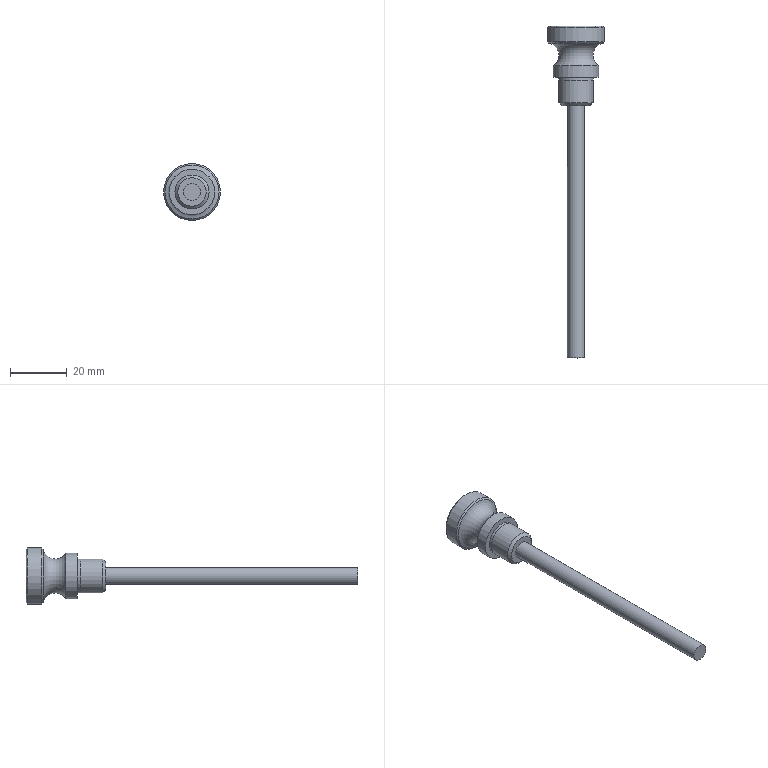Part | NX | 1 solid | 14 faces | box 20.002 x 116.72 x 20.002 mm | volume 7452 mm3 | plane 5 | cone 4 | cylinder 4 | torus 1 | commonest cylinder face diameters 5.996 x1 12.002 x1 16.002 x1 20.002 x1
STEP:
#1=CARTESIAN_POINT('',(9.502,116.719,0.));
#2=VERTEX_POINT('',#1);
#3=CARTESIAN_POINT('',(0.000965,116.72,0.));
#4=DIRECTION('',(-0.000008268,-1.,0.));
#5=DIRECTION('',(1.,-0.000008268,0.));
#6=AXIS2_PLACEMENT_3D('',#3,#4,#5);
#7=CIRCLE('',#6,9.501);
#8=EDGE_CURVE('',#2,#2,#7,.T.);
#9=ORIENTED_EDGE('',*,*,#8,.F.);
#10=EDGE_LOOP('',(#9));
#11=FACE_OUTER_BOUND('',#10,.T.);
#12=CARTESIAN_POINT('',(-9.5,116.72,0.));
#13=DIRECTION('',(0.000008268,1.,0.));
#14=DIRECTION('',(1.,-0.000008268,0.));
#15=AXIS2_PLACEMENT_3D('',#12,#13,#14);
#16=PLANE('',#15);
#17=ADVANCED_FACE('',(#11),#16,.T.);
#18=ORIENTED_EDGE('',*,*,#8,.T.);
#19=EDGE_LOOP('',(#18));
#20=FACE_BOUND('',#19,.T.);
#21=CARTESIAN_POINT('',(10.002,116.219,0.));
#22=VERTEX_POINT('',#21);
#23=CARTESIAN_POINT('',(0.0009609,116.22,0.));
#24=DIRECTION('',(-0.000008268,-1.,0.));
#25=DIRECTION('',(1.,-0.000008268,0.));
#26=AXIS2_PLACEMENT_3D('',#23,#24,#25);
#27=CIRCLE('',#26,10.001);
#28=EDGE_CURVE('',#22,#22,#27,.T.);
#29=ORIENTED_EDGE('',*,*,#28,.F.);
#30=EDGE_LOOP('',(#29));
#31=FACE_BOUND('',#30,.T.);
#32=CARTESIAN_POINT('',(0.0009609,116.22,0.));
#33=DIRECTION('',(-0.000008268,-1.,0.));
#34=DIRECTION('',(-1.,0.000008268,0.));
#35=AXIS2_PLACEMENT_3D('',#32,#33,#34);
#36=CONICAL_SURFACE('',#35,10.001,45.);
#37=ADVANCED_FACE('',(#20,#31),#36,.T.);
#38=ORIENTED_EDGE('',*,*,#28,.T.);
#39=EDGE_LOOP('',(#38));
#40=FACE_BOUND('',#39,.T.);
#41=CARTESIAN_POINT('',(10.002,111.219,0.));
#42=VERTEX_POINT('',#41);
#43=CARTESIAN_POINT('',(0.0009195,111.22,0.));
#44=DIRECTION('',(-0.000008268,-1.,0.));
#45=DIRECTION('',(1.,-0.000008268,0.));
#46=AXIS2_PLACEMENT_3D('',#43,#44,#45);
#47=CIRCLE('',#46,10.001);
#48=EDGE_CURVE('',#42,#42,#47,.T.);
#49=ORIENTED_EDGE('',*,*,#48,.F.);
#50=EDGE_LOOP('',(#49));
#51=FACE_BOUND('',#50,.T.);
#52=CARTESIAN_POINT('',(-0.00004139,-5.006,0.));
#53=DIRECTION('',(-0.000008268,-1.,0.));
#54=DIRECTION('',(-1.,0.000008268,0.));
#55=AXIS2_PLACEMENT_3D('',#52,#53,#54);
#56=CYLINDRICAL_SURFACE('',#55,10.001);
#57=ADVANCED_FACE('',(#40,#51),#56,.T.);
#58=ORIENTED_EDGE('',*,*,#48,.T.);
#59=EDGE_LOOP('',(#58));
#60=FACE_BOUND('',#59,.T.);
#61=CARTESIAN_POINT('',(9.502,110.719,0.));
#62=VERTEX_POINT('',#61);
#63=CARTESIAN_POINT('',(0.0009154,110.72,0.));
#64=DIRECTION('',(-0.000008268,-1.,0.));
#65=DIRECTION('',(1.,-0.000008268,0.));
#66=AXIS2_PLACEMENT_3D('',#63,#64,#65);
#67=CIRCLE('',#66,9.501);
#68=EDGE_CURVE('',#62,#62,#67,.T.);
#69=ORIENTED_EDGE('',*,*,#68,.F.);
#70=EDGE_LOOP('',(#69));
#71=FACE_BOUND('',#70,.T.);
#72=CARTESIAN_POINT('',(0.0009154,110.72,0.));
#73=DIRECTION('',(0.000008268,1.,0.));
#74=DIRECTION('',(1.,-0.000008268,0.));
#75=AXIS2_PLACEMENT_3D('',#72,#73,#74);
#76=CONICAL_SURFACE('',#75,9.501,45.);
#77=ADVANCED_FACE('',(#60,#71),#76,.T.);
#78=ORIENTED_EDGE('',*,*,#68,.T.);
#79=EDGE_LOOP('',(#78));
#80=FACE_BOUND('',#79,.T.);
#81=CARTESIAN_POINT('',(8.002,102.719,0.));
#82=VERTEX_POINT('',#81);
#83=CARTESIAN_POINT('',(0.0008493,102.72,0.));
#84=DIRECTION('',(-0.000008268,-1.,0.));
#85=DIRECTION('',(1.,-0.000008268,0.));
#86=AXIS2_PLACEMENT_3D('',#83,#84,#85);
#87=CIRCLE('',#86,8.001);
#88=EDGE_CURVE('',#82,#82,#87,.T.);
#89=ORIENTED_EDGE('',*,*,#88,.F.);
#90=EDGE_LOOP('',(#89));
#91=FACE_BOUND('',#90,.T.);
#92=CARTESIAN_POINT('',(0.0008798,106.411,0.));
#93=DIRECTION('',(-0.000008268,-1.,0.));
#94=DIRECTION('',(-1.,0.000008268,0.));
#95=AXIS2_PLACEMENT_3D('',#92,#93,#94);
#96=TOROIDAL_SURFACE('',#95,10.396,4.401);
#97=ADVANCED_FACE('',(#80,#91),#96,.F.);
#98=ORIENTED_EDGE('',*,*,#88,.T.);
#99=EDGE_LOOP('',(#98));
#100=FACE_BOUND('',#99,.T.);
#101=CARTESIAN_POINT('',(8.002,98.719,0.));
#102=VERTEX_POINT('',#101);
#103=CARTESIAN_POINT('',(0.0008162,98.72,0.));
#104=DIRECTION('',(-0.000008268,-1.,0.));
#105=DIRECTION('',(1.,-0.000008268,0.));
#106=AXIS2_PLACEMENT_3D('',#103,#104,#105);
#107=CIRCLE('',#106,8.001);
#108=EDGE_CURVE('',#102,#102,#107,.T.);
#109=ORIENTED_EDGE('',*,*,#108,.F.);
#110=EDGE_LOOP('',(#109));
#111=FACE_BOUND('',#110,.T.);
#112=CARTESIAN_POINT('',(-0.00004139,-5.006,0.));
#113=DIRECTION('',(-0.000008268,-1.,0.));
#114=DIRECTION('',(-1.,0.000008268,0.));
#115=AXIS2_PLACEMENT_3D('',#112,#113,#114);
#116=CYLINDRICAL_SURFACE('',#115,8.001);
#117=ADVANCED_FACE('',(#100,#111),#116,.T.);
#118=ORIENTED_EDGE('',*,*,#108,.T.);
#119=EDGE_LOOP('',(#118));
#120=FACE_BOUND('',#119,.T.);
#121=CARTESIAN_POINT('',(5.997,98.72,0.));
#122=VERTEX_POINT('',#121);
#123=CARTESIAN_POINT('',(0.0008162,98.72,0.));
#124=DIRECTION('',(-0.000008268,-1.,0.));
#125=DIRECTION('',(1.,-0.000008268,0.));
#126=AXIS2_PLACEMENT_3D('',#123,#124,#125);
#127=CIRCLE('',#126,5.996);
#128=EDGE_CURVE('',#122,#122,#127,.T.);
#129=ORIENTED_EDGE('',*,*,#128,.F.);
#130=EDGE_LOOP('',(#129));
#131=FACE_BOUND('',#130,.T.);
#132=CARTESIAN_POINT('',(-5.995,98.72,0.));
#133=DIRECTION('',(-0.000008268,-1.,0.));
#134=DIRECTION('',(-1.,0.000008268,0.));
#135=AXIS2_PLACEMENT_3D('',#132,#133,#134);
#136=PLANE('',#135);
#137=ADVANCED_FACE('',(#120,#131),#136,.T.);
#138=ORIENTED_EDGE('',*,*,#128,.T.);
#139=EDGE_LOOP('',(#138));
#140=FACE_BOUND('',#139,.T.);
#141=CARTESIAN_POINT('',(5.998,97.72,0.));
#142=VERTEX_POINT('',#141);
#143=CARTESIAN_POINT('',(0.0008079,97.72,0.));
#144=DIRECTION('',(-0.000008268,-1.,0.));
#145=DIRECTION('',(1.,-0.000008268,0.));
#146=AXIS2_PLACEMENT_3D('',#143,#144,#145);
#147=CIRCLE('',#146,5.997);
#148=EDGE_CURVE('',#142,#142,#147,.T.);
#149=ORIENTED_EDGE('',*,*,#148,.F.);
#150=EDGE_LOOP('',(#149));
#151=FACE_BOUND('',#150,.T.);
#152=CARTESIAN_POINT('',(0.0008079,97.72,0.));
#153=DIRECTION('',(-0.000008268,-1.,0.));
#154=DIRECTION('',(-1.,0.000008268,0.));
#155=AXIS2_PLACEMENT_3D('',#152,#153,#154);
#156=CONICAL_SURFACE('',#155,5.997,0.04501);
#157=ADVANCED_FACE('',(#140,#151),#156,.T.);
#158=ORIENTED_EDGE('',*,*,#148,.T.);
#159=EDGE_LOOP('',(#158));
#160=FACE_BOUND('',#159,.T.);
#161=CARTESIAN_POINT('',(6.002,97.72,0.));
#162=VERTEX_POINT('',#161);
#163=CARTESIAN_POINT('',(0.0008079,97.72,0.));
#164=DIRECTION('',(-0.000008268,-1.,0.));
#165=DIRECTION('',(1.,-0.000008268,0.));
#166=AXIS2_PLACEMENT_3D('',#163,#164,#165);
#167=CIRCLE('',#166,6.001);
#168=EDGE_CURVE('',#162,#162,#167,.T.);
#169=ORIENTED_EDGE('',*,*,#168,.F.);
#170=EDGE_LOOP('',(#169));
#171=FACE_BOUND('',#170,.T.);
#172=CARTESIAN_POINT('',(0.0008079,97.72,0.));
#173=DIRECTION('',(-0.000008268,-1.,0.));
#174=DIRECTION('',(-1.,0.000008268,0.));
#175=AXIS2_PLACEMENT_3D('',#172,#173,#174);
#176=PLANE('',#175);
#177=ADVANCED_FACE('',(#160,#171),#176,.F.);
#178=CARTESIAN_POINT('',(2.998,-0.00002479,0.));
#179=VERTEX_POINT('',#178);
#180=CARTESIAN_POINT('',(0.,0.,0.));
#181=DIRECTION('',(-0.000008268,-1.,0.));
#182=DIRECTION('',(1.,-0.000008268,0.));
#183=AXIS2_PLACEMENT_3D('',#180,#181,#182);
#184=CIRCLE('',#183,2.998);
#185=EDGE_CURVE('',#179,#179,#184,.T.);
#186=ORIENTED_EDGE('',*,*,#185,.T.);
#187=EDGE_LOOP('',(#186));
#188=FACE_OUTER_BOUND('',#187,.T.);
#189=CARTESIAN_POINT('',(-2.998,0.00002479,0.));
#190=DIRECTION('',(0.000008268,1.,0.));
#191=DIRECTION('',(1.,-0.000008268,0.));
#192=AXIS2_PLACEMENT_3D('',#189,#190,#191);
#193=PLANE('',#192);
#194=ADVANCED_FACE('',(#188),#193,.F.);
#195=ORIENTED_EDGE('',*,*,#185,.F.);
#196=EDGE_LOOP('',(#195));
#197=FACE_BOUND('',#196,.T.);
#198=CARTESIAN_POINT('',(2.999,88.72,0.));
#199=VERTEX_POINT('',#198);
#200=CARTESIAN_POINT('',(0.0007335,88.72,0.));
#201=DIRECTION('',(-0.000008268,-1.,0.));
#202=DIRECTION('',(1.,-0.000008268,0.));
#203=AXIS2_PLACEMENT_3D('',#200,#201,#202);
#204=CIRCLE('',#203,2.998);
#205=EDGE_CURVE('',#199,#199,#204,.T.);
#206=ORIENTED_EDGE('',*,*,#205,.T.);
#207=EDGE_LOOP('',(#206));
#208=FACE_BOUND('',#207,.T.);
#209=CARTESIAN_POINT('',(-0.00004139,-5.006,0.));
#210=DIRECTION('',(-0.000008268,-1.,0.));
#211=DIRECTION('',(-1.,0.000008268,0.));
#212=AXIS2_PLACEMENT_3D('',#209,#210,#211);
#213=CYLINDRICAL_SURFACE('',#212,2.998);
#214=ADVANCED_FACE('',(#197,#208),#213,.T.);
#215=ORIENTED_EDGE('',*,*,#205,.F.);
#216=EDGE_LOOP('',(#215));
#217=FACE_BOUND('',#216,.T.);
#218=CARTESIAN_POINT('',(5.002,88.72,0.));
#219=VERTEX_POINT('',#218);
#220=CARTESIAN_POINT('',(0.0007335,88.72,0.));
#221=DIRECTION('',(-0.000008268,-1.,0.));
#222=DIRECTION('',(1.,-0.000008268,0.));
#223=AXIS2_PLACEMENT_3D('',#220,#221,#222);
#224=CIRCLE('',#223,5.001);
#225=EDGE_CURVE('',#219,#219,#224,.T.);
#226=ORIENTED_EDGE('',*,*,#225,.T.);
#227=EDGE_LOOP('',(#226));
#228=FACE_BOUND('',#227,.T.);
#229=CARTESIAN_POINT('',(-5.,88.72,0.));
#230=DIRECTION('',(0.000008268,1.,0.));
#231=DIRECTION('',(1.,-0.000008268,0.));
#232=AXIS2_PLACEMENT_3D('',#229,#230,#231);
#233=PLANE('',#232);
#234=ADVANCED_FACE('',(#217,#228),#233,.F.);
#235=ORIENTED_EDGE('',*,*,#225,.F.);
#236=EDGE_LOOP('',(#235));
#237=FACE_BOUND('',#236,.T.);
#238=CARTESIAN_POINT('',(6.002,89.72,0.));
#239=VERTEX_POINT('',#238);
#240=CARTESIAN_POINT('',(0.0007418,89.72,0.));
#241=DIRECTION('',(-0.000008268,-1.,0.));
#242=DIRECTION('',(1.,-0.000008268,0.));
#243=AXIS2_PLACEMENT_3D('',#240,#241,#242);
#244=CIRCLE('',#243,6.001);
#245=EDGE_CURVE('',#239,#239,#244,.T.);
#246=ORIENTED_EDGE('',*,*,#245,.T.);
#247=EDGE_LOOP('',(#246));
#248=FACE_BOUND('',#247,.T.);
#249=CARTESIAN_POINT('',(0.0007418,89.72,0.));
#250=DIRECTION('',(0.000008268,1.,0.));
#251=DIRECTION('',(1.,-0.000008268,0.));
#252=AXIS2_PLACEMENT_3D('',#249,#250,#251);
#253=CONICAL_SURFACE('',#252,6.001,45.);
#254=ADVANCED_FACE('',(#237,#248),#253,.T.);
#255=ORIENTED_EDGE('',*,*,#245,.F.);
#256=EDGE_LOOP('',(#255));
#257=FACE_BOUND('',#256,.T.);
#258=ORIENTED_EDGE('',*,*,#168,.T.);
#259=EDGE_LOOP('',(#258));
#260=FACE_BOUND('',#259,.T.);
#261=CARTESIAN_POINT('',(-0.00004139,-5.006,0.));
#262=DIRECTION('',(-0.000008268,-1.,0.));
#263=DIRECTION('',(-1.,0.000008268,0.));
#264=AXIS2_PLACEMENT_3D('',#261,#262,#263);
#265=CYLINDRICAL_SURFACE('',#264,6.001);
#266=ADVANCED_FACE('',(#257,#260),#265,.T.);
#267=CLOSED_SHELL('',(#17,#37,#57,#77,#97,#117,#137,#157,#177,#194,#214,#234,#254,#266));
#268=MANIFOLD_SOLID_BREP('',#267);
#269=(LENGTH_UNIT()NAMED_UNIT(*)SI_UNIT(.MILLI.,.METRE.));
#270=UNCERTAINTY_MEASURE_WITH_UNIT(LENGTH_MEASURE(0.00002),#269,'','');
#271=(NAMED_UNIT(*)PLANE_ANGLE_UNIT()SI_UNIT($,.RADIAN.));
#272=PLANE_ANGLE_MEASURE_WITH_UNIT(PLANE_ANGLE_MEASURE(0.01745),#271);
#273=DIMENSIONAL_EXPONENTS(0.,0.,0.,0.,0.,0.,0.);
#274=(CONVERSION_BASED_UNIT('DEGREE',#272)NAMED_UNIT(#273)PLANE_ANGLE_UNIT());
#275=(NAMED_UNIT(*)SI_UNIT($,.STERADIAN.)SOLID_ANGLE_UNIT());
#276=(GEOMETRIC_REPRESENTATION_CONTEXT(3)GLOBAL_UNCERTAINTY_ASSIGNED_CONTEXT((#270))GLOBAL_UNIT_ASSIGNED_CONTEXT((#269,#274,#275))REPRESENTATION_CONTEXT('',''));
#277=ADVANCED_BREP_SHAPE_REPRESENTATION('',(#268),#276);